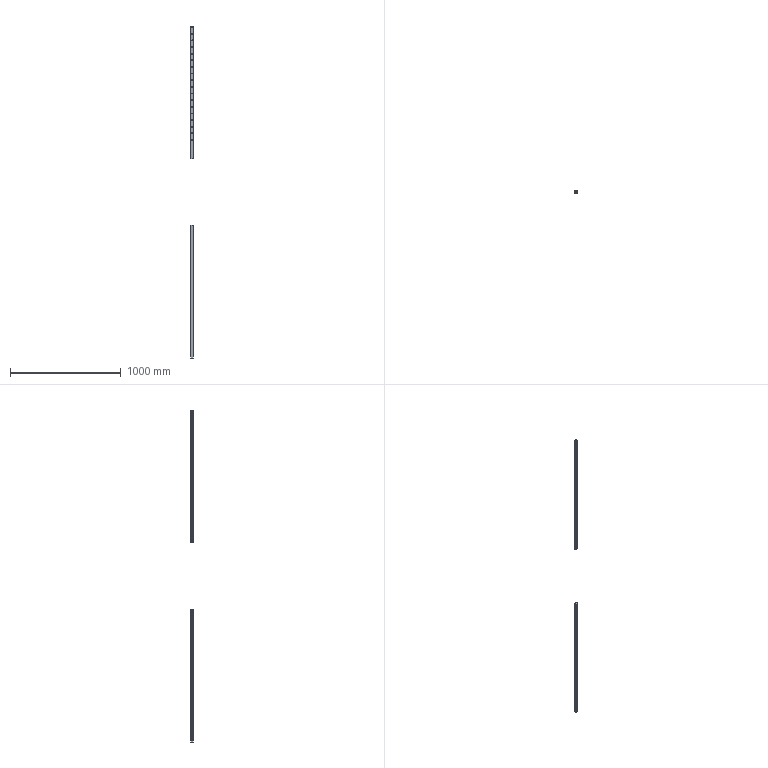Part | SolidWorks | features Chamfer 1, Extrusion 1, HoleWzd 1, ICE 1, LPattern 1 | 2 solids | 146 faces | box 23.859 x 22 x 3000 mm | volume 1088729 mm3 | cylinder 92 | plane 54 | commonest cylinder face diameters 7 x36 11 x36 2.933 x20